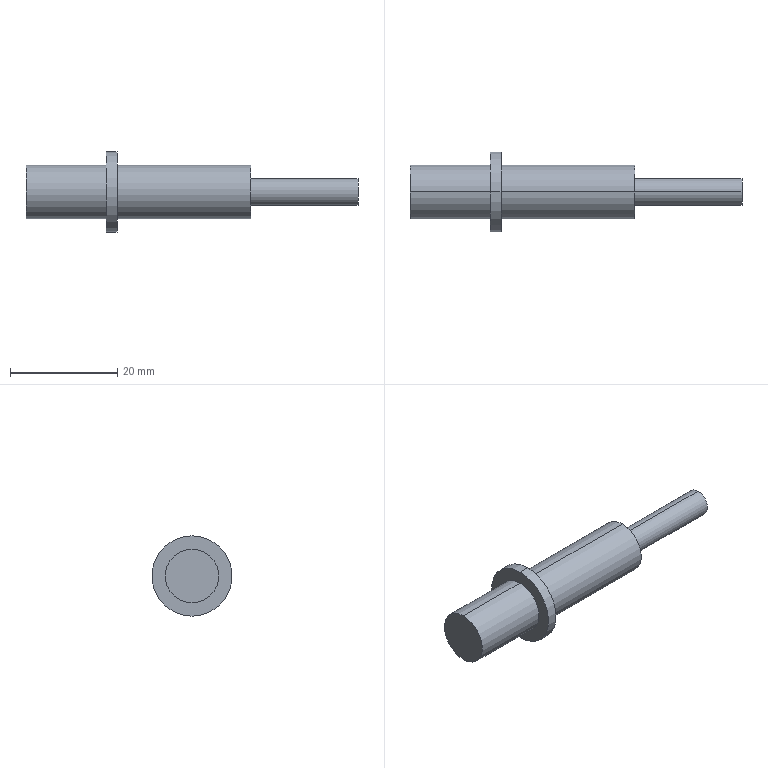Part | SolidWorks | features ICE 3, Extrusion 1 | 1 solid | 13 faces | box 62 x 15 x 15 mm | volume 3888 mm3 | cylinder 8 | plane 5 | commonest cylinder face diameters 10 x4 5 x2 15 x2
STEP:
#1=CARTESIAN_POINT('',(-42.,0.,5.));
#2=VERTEX_POINT('',#1);
#3=CARTESIAN_POINT('',(-42.,0.,-5.));
#4=VERTEX_POINT('',#3);
#5=CARTESIAN_POINT('',(-42.,0.,0.));
#6=DIRECTION('',(-1.,0.,0.));
#7=DIRECTION('',(0.,0.,1.));
#8=AXIS2_PLACEMENT_3D('',#5,#6,#7);
#9=CIRCLE('',#8,5.);
#10=EDGE_CURVE('',#2,#4,#9,.T.);
#11=ORIENTED_EDGE('',*,*,#10,.F.);
#12=CARTESIAN_POINT('',(-27.,0.,5.));
#13=VERTEX_POINT('',#12);
#14=CARTESIAN_POINT('',(-42.,0.,5.));
#15=DIRECTION('',(1.,0.,0.));
#16=VECTOR('',#15,1000.);
#17=LINE('',#14,#16);
#18=EDGE_CURVE('',#2,#13,#17,.T.);
#19=ORIENTED_EDGE('',*,*,#18,.T.);
#20=CARTESIAN_POINT('',(-27.,0.,-5.));
#21=VERTEX_POINT('',#20);
#22=CARTESIAN_POINT('',(-27.,0.,0.));
#23=DIRECTION('',(-1.,0.,0.));
#24=DIRECTION('',(0.,0.,1.));
#25=AXIS2_PLACEMENT_3D('',#22,#23,#24);
#26=CIRCLE('',#25,5.);
#27=EDGE_CURVE('',#13,#21,#26,.T.);
#28=ORIENTED_EDGE('',*,*,#27,.T.);
#29=CARTESIAN_POINT('',(-42.,0.,-5.));
#30=DIRECTION('',(1.,0.,0.));
#31=VECTOR('',#30,1000.);
#32=LINE('',#29,#31);
#33=EDGE_CURVE('',#4,#21,#32,.T.);
#34=ORIENTED_EDGE('',*,*,#33,.F.);
#35=EDGE_LOOP('',(#11,#19,#28,#34));
#36=FACE_OUTER_BOUND('',#35,.T.);
#37=CARTESIAN_POINT('',(-42.,0.,0.));
#38=DIRECTION('',(1.,0.,0.));
#39=DIRECTION('',(0.,0.,-1.));
#40=AXIS2_PLACEMENT_3D('',#37,#38,#39);
#41=CYLINDRICAL_SURFACE('',#40,5.);
#42=ADVANCED_FACE('',(#36),#41,.T.);
#43=CARTESIAN_POINT('',(-27.,0.,7.5));
#44=VERTEX_POINT('',#43);
#45=CARTESIAN_POINT('',(-27.,0.,-7.5));
#46=VERTEX_POINT('',#45);
#47=CARTESIAN_POINT('',(-27.,0.,0.));
#48=DIRECTION('',(-1.,0.,0.));
#49=DIRECTION('',(0.,0.,1.));
#50=AXIS2_PLACEMENT_3D('',#47,#48,#49);
#51=CIRCLE('',#50,7.5);
#52=EDGE_CURVE('',#44,#46,#51,.T.);
#53=ORIENTED_EDGE('',*,*,#52,.F.);
#54=CARTESIAN_POINT('',(-25.,0.,7.5));
#55=VERTEX_POINT('',#54);
#56=CARTESIAN_POINT('',(-27.,0.,7.5));
#57=DIRECTION('',(1.,0.,0.));
#58=VECTOR('',#57,1000.);
#59=LINE('',#56,#58);
#60=EDGE_CURVE('',#44,#55,#59,.T.);
#61=ORIENTED_EDGE('',*,*,#60,.T.);
#62=CARTESIAN_POINT('',(-25.,0.,-7.5));
#63=VERTEX_POINT('',#62);
#64=CARTESIAN_POINT('',(-25.,0.,0.));
#65=DIRECTION('',(-1.,0.,0.));
#66=DIRECTION('',(0.,0.,1.));
#67=AXIS2_PLACEMENT_3D('',#64,#65,#66);
#68=CIRCLE('',#67,7.5);
#69=EDGE_CURVE('',#55,#63,#68,.T.);
#70=ORIENTED_EDGE('',*,*,#69,.T.);
#71=CARTESIAN_POINT('',(-27.,0.,-7.5));
#72=DIRECTION('',(1.,0.,0.));
#73=VECTOR('',#72,1000.);
#74=LINE('',#71,#73);
#75=EDGE_CURVE('',#46,#63,#74,.T.);
#76=ORIENTED_EDGE('',*,*,#75,.F.);
#77=EDGE_LOOP('',(#53,#61,#70,#76));
#78=FACE_OUTER_BOUND('',#77,.T.);
#79=CARTESIAN_POINT('',(-27.,0.,0.));
#80=DIRECTION('',(1.,0.,0.));
#81=DIRECTION('',(0.,0.,-1.));
#82=AXIS2_PLACEMENT_3D('',#79,#80,#81);
#83=CYLINDRICAL_SURFACE('',#82,7.5);
#84=ADVANCED_FACE('',(#78),#83,.T.);
#85=CARTESIAN_POINT('',(-25.,0.,5.));
#86=VERTEX_POINT('',#85);
#87=CARTESIAN_POINT('',(-25.,0.,-5.));
#88=VERTEX_POINT('',#87);
#89=CARTESIAN_POINT('',(-25.,0.,0.));
#90=DIRECTION('',(-1.,0.,0.));
#91=DIRECTION('',(0.,0.,1.));
#92=AXIS2_PLACEMENT_3D('',#89,#90,#91);
#93=CIRCLE('',#92,5.);
#94=EDGE_CURVE('',#86,#88,#93,.T.);
#95=ORIENTED_EDGE('',*,*,#94,.F.);
#96=CARTESIAN_POINT('',(0.,0.,5.));
#97=VERTEX_POINT('',#96);
#98=CARTESIAN_POINT('',(-25.,0.,5.));
#99=DIRECTION('',(1.,0.,0.));
#100=VECTOR('',#99,1000.);
#101=LINE('',#98,#100);
#102=EDGE_CURVE('',#86,#97,#101,.T.);
#103=ORIENTED_EDGE('',*,*,#102,.T.);
#104=CARTESIAN_POINT('',(0.,0.,-5.));
#105=VERTEX_POINT('',#104);
#106=CARTESIAN_POINT('',(0.,0.,0.));
#107=DIRECTION('',(-1.,0.,0.));
#108=DIRECTION('',(0.,0.,1.));
#109=AXIS2_PLACEMENT_3D('',#106,#107,#108);
#110=CIRCLE('',#109,5.);
#111=EDGE_CURVE('',#97,#105,#110,.T.);
#112=ORIENTED_EDGE('',*,*,#111,.T.);
#113=CARTESIAN_POINT('',(-25.,0.,-5.));
#114=DIRECTION('',(1.,0.,0.));
#115=VECTOR('',#114,1000.);
#116=LINE('',#113,#115);
#117=EDGE_CURVE('',#88,#105,#116,.T.);
#118=ORIENTED_EDGE('',*,*,#117,.F.);
#119=EDGE_LOOP('',(#95,#103,#112,#118));
#120=FACE_OUTER_BOUND('',#119,.T.);
#121=CARTESIAN_POINT('',(-25.,0.,0.));
#122=DIRECTION('',(1.,0.,0.));
#123=DIRECTION('',(0.,0.,-1.));
#124=AXIS2_PLACEMENT_3D('',#121,#122,#123);
#125=CYLINDRICAL_SURFACE('',#124,5.);
#126=ADVANCED_FACE('',(#120),#125,.T.);
#127=CARTESIAN_POINT('',(20.,0.,-2.5));
#128=VERTEX_POINT('',#127);
#129=CARTESIAN_POINT('',(20.,0.,2.5));
#130=VERTEX_POINT('',#129);
#131=CARTESIAN_POINT('',(20.,0.,0.));
#132=DIRECTION('',(1.,0.,0.));
#133=DIRECTION('',(0.,0.,-1.));
#134=AXIS2_PLACEMENT_3D('',#131,#132,#133);
#135=CIRCLE('',#134,2.5);
#136=EDGE_CURVE('',#128,#130,#135,.T.);
#137=ORIENTED_EDGE('',*,*,#136,.F.);
#138=CARTESIAN_POINT('',(0.,0.,-2.5));
#139=VERTEX_POINT('',#138);
#140=CARTESIAN_POINT('',(20.,0.,-2.5));
#141=DIRECTION('',(-1.,0.,0.));
#142=VECTOR('',#141,1000.);
#143=LINE('',#140,#142);
#144=EDGE_CURVE('',#128,#139,#143,.T.);
#145=ORIENTED_EDGE('',*,*,#144,.T.);
#146=CARTESIAN_POINT('',(0.,0.,2.5));
#147=VERTEX_POINT('',#146);
#148=CARTESIAN_POINT('',(0.,0.,0.));
#149=DIRECTION('',(1.,0.,0.));
#150=DIRECTION('',(0.,0.,-1.));
#151=AXIS2_PLACEMENT_3D('',#148,#149,#150);
#152=CIRCLE('',#151,2.5);
#153=EDGE_CURVE('',#139,#147,#152,.T.);
#154=ORIENTED_EDGE('',*,*,#153,.T.);
#155=CARTESIAN_POINT('',(20.,0.,2.5));
#156=DIRECTION('',(-1.,0.,0.));
#157=VECTOR('',#156,1000.);
#158=LINE('',#155,#157);
#159=EDGE_CURVE('',#130,#147,#158,.T.);
#160=ORIENTED_EDGE('',*,*,#159,.F.);
#161=EDGE_LOOP('',(#137,#145,#154,#160));
#162=FACE_OUTER_BOUND('',#161,.T.);
#163=CARTESIAN_POINT('',(20.,0.,0.));
#164=DIRECTION('',(-1.,0.,0.));
#165=DIRECTION('',(0.,0.,1.));
#166=AXIS2_PLACEMENT_3D('',#163,#164,#165);
#167=CYLINDRICAL_SURFACE('',#166,2.5);
#168=ADVANCED_FACE('',(#162),#167,.T.);
#169=ORIENTED_EDGE('',*,*,#144,.F.);
#170=CARTESIAN_POINT('',(20.,0.,0.));
#171=DIRECTION('',(1.,0.,0.));
#172=DIRECTION('',(0.,0.,-1.));
#173=AXIS2_PLACEMENT_3D('',#170,#171,#172);
#174=CIRCLE('',#173,2.5);
#175=EDGE_CURVE('',#130,#128,#174,.T.);
#176=ORIENTED_EDGE('',*,*,#175,.F.);
#177=ORIENTED_EDGE('',*,*,#159,.T.);
#178=CARTESIAN_POINT('',(0.,0.,0.));
#179=DIRECTION('',(1.,0.,0.));
#180=DIRECTION('',(0.,0.,-1.));
#181=AXIS2_PLACEMENT_3D('',#178,#179,#180);
#182=CIRCLE('',#181,2.5);
#183=EDGE_CURVE('',#147,#139,#182,.T.);
#184=ORIENTED_EDGE('',*,*,#183,.T.);
#185=EDGE_LOOP('',(#169,#176,#177,#184));
#186=FACE_OUTER_BOUND('',#185,.T.);
#187=CARTESIAN_POINT('',(20.,0.,0.));
#188=DIRECTION('',(-1.,0.,0.));
#189=DIRECTION('',(0.,0.,1.));
#190=AXIS2_PLACEMENT_3D('',#187,#188,#189);
#191=CYLINDRICAL_SURFACE('',#190,2.5);
#192=ADVANCED_FACE('',(#186),#191,.T.);
#193=ORIENTED_EDGE('',*,*,#175,.T.);
#194=ORIENTED_EDGE('',*,*,#136,.T.);
#195=EDGE_LOOP('',(#193,#194));
#196=FACE_OUTER_BOUND('',#195,.T.);
#197=CARTESIAN_POINT('',(20.,0.,0.));
#198=DIRECTION('',(1.,0.,0.));
#199=DIRECTION('',(0.,0.,-1.));
#200=AXIS2_PLACEMENT_3D('',#197,#198,#199);
#201=PLANE('',#200);
#202=ADVANCED_FACE('',(#196),#201,.T.);
#203=ORIENTED_EDGE('',*,*,#102,.F.);
#204=CARTESIAN_POINT('',(-25.,0.,0.));
#205=DIRECTION('',(-1.,0.,0.));
#206=DIRECTION('',(0.,0.,1.));
#207=AXIS2_PLACEMENT_3D('',#204,#205,#206);
#208=CIRCLE('',#207,5.);
#209=EDGE_CURVE('',#88,#86,#208,.T.);
#210=ORIENTED_EDGE('',*,*,#209,.F.);
#211=ORIENTED_EDGE('',*,*,#117,.T.);
#212=CARTESIAN_POINT('',(0.,0.,0.));
#213=DIRECTION('',(-1.,0.,0.));
#214=DIRECTION('',(0.,0.,1.));
#215=AXIS2_PLACEMENT_3D('',#212,#213,#214);
#216=CIRCLE('',#215,5.);
#217=EDGE_CURVE('',#105,#97,#216,.T.);
#218=ORIENTED_EDGE('',*,*,#217,.T.);
#219=EDGE_LOOP('',(#203,#210,#211,#218));
#220=FACE_OUTER_BOUND('',#219,.T.);
#221=CARTESIAN_POINT('',(-25.,0.,0.));
#222=DIRECTION('',(1.,0.,0.));
#223=DIRECTION('',(0.,0.,-1.));
#224=AXIS2_PLACEMENT_3D('',#221,#222,#223);
#225=CYLINDRICAL_SURFACE('',#224,5.);
#226=ADVANCED_FACE('',(#220),#225,.T.);
#227=ORIENTED_EDGE('',*,*,#183,.F.);
#228=ORIENTED_EDGE('',*,*,#153,.F.);
#229=EDGE_LOOP('',(#227,#228));
#230=FACE_BOUND('',#229,.T.);
#231=ORIENTED_EDGE('',*,*,#217,.F.);
#232=ORIENTED_EDGE('',*,*,#111,.F.);
#233=EDGE_LOOP('',(#231,#232));
#234=FACE_OUTER_BOUND('',#233,.T.);
#235=CARTESIAN_POINT('',(0.,0.,0.));
#236=DIRECTION('',(-1.,0.,0.));
#237=DIRECTION('',(0.,0.,1.));
#238=AXIS2_PLACEMENT_3D('',#235,#236,#237);
#239=PLANE('',#238);
#240=ADVANCED_FACE('',(#230,#234),#239,.F.);
#241=ORIENTED_EDGE('',*,*,#60,.F.);
#242=CARTESIAN_POINT('',(-27.,0.,0.));
#243=DIRECTION('',(-1.,0.,0.));
#244=DIRECTION('',(0.,0.,1.));
#245=AXIS2_PLACEMENT_3D('',#242,#243,#244);
#246=CIRCLE('',#245,7.5);
#247=EDGE_CURVE('',#46,#44,#246,.T.);
#248=ORIENTED_EDGE('',*,*,#247,.F.);
#249=ORIENTED_EDGE('',*,*,#75,.T.);
#250=CARTESIAN_POINT('',(-25.,0.,0.));
#251=DIRECTION('',(-1.,0.,0.));
#252=DIRECTION('',(0.,0.,1.));
#253=AXIS2_PLACEMENT_3D('',#250,#251,#252);
#254=CIRCLE('',#253,7.5);
#255=EDGE_CURVE('',#63,#55,#254,.T.);
#256=ORIENTED_EDGE('',*,*,#255,.T.);
#257=EDGE_LOOP('',(#241,#248,#249,#256));
#258=FACE_OUTER_BOUND('',#257,.T.);
#259=CARTESIAN_POINT('',(-27.,0.,0.));
#260=DIRECTION('',(1.,0.,0.));
#261=DIRECTION('',(0.,0.,-1.));
#262=AXIS2_PLACEMENT_3D('',#259,#260,#261);
#263=CYLINDRICAL_SURFACE('',#262,7.5);
#264=ADVANCED_FACE('',(#258),#263,.T.);
#265=CARTESIAN_POINT('',(-27.,0.,0.));
#266=DIRECTION('',(-1.,0.,0.));
#267=DIRECTION('',(0.,0.,1.));
#268=AXIS2_PLACEMENT_3D('',#265,#266,#267);
#269=CIRCLE('',#268,5.);
#270=EDGE_CURVE('',#21,#13,#269,.T.);
#271=ORIENTED_EDGE('',*,*,#270,.F.);
#272=ORIENTED_EDGE('',*,*,#27,.F.);
#273=EDGE_LOOP('',(#271,#272));
#274=FACE_BOUND('',#273,.T.);
#275=ORIENTED_EDGE('',*,*,#247,.T.);
#276=ORIENTED_EDGE('',*,*,#52,.T.);
#277=EDGE_LOOP('',(#275,#276));
#278=FACE_OUTER_BOUND('',#277,.T.);
#279=CARTESIAN_POINT('',(-27.,0.,0.));
#280=DIRECTION('',(-1.,0.,0.));
#281=DIRECTION('',(0.,0.,1.));
#282=AXIS2_PLACEMENT_3D('',#279,#280,#281);
#283=PLANE('',#282);
#284=ADVANCED_FACE('',(#274,#278),#283,.T.);
#285=ORIENTED_EDGE('',*,*,#209,.T.);
#286=ORIENTED_EDGE('',*,*,#94,.T.);
#287=EDGE_LOOP('',(#285,#286));
#288=FACE_BOUND('',#287,.T.);
#289=ORIENTED_EDGE('',*,*,#255,.F.);
#290=ORIENTED_EDGE('',*,*,#69,.F.);
#291=EDGE_LOOP('',(#289,#290));
#292=FACE_OUTER_BOUND('',#291,.T.);
#293=CARTESIAN_POINT('',(-25.,0.,0.));
#294=DIRECTION('',(-1.,0.,0.));
#295=DIRECTION('',(0.,0.,1.));
#296=AXIS2_PLACEMENT_3D('',#293,#294,#295);
#297=PLANE('',#296);
#298=ADVANCED_FACE('',(#288,#292),#297,.F.);
#299=ORIENTED_EDGE('',*,*,#18,.F.);
#300=CARTESIAN_POINT('',(-42.,0.,0.));
#301=DIRECTION('',(-1.,0.,0.));
#302=DIRECTION('',(0.,0.,1.));
#303=AXIS2_PLACEMENT_3D('',#300,#301,#302);
#304=CIRCLE('',#303,5.);
#305=EDGE_CURVE('',#4,#2,#304,.T.);
#306=ORIENTED_EDGE('',*,*,#305,.F.);
#307=ORIENTED_EDGE('',*,*,#33,.T.);
#308=ORIENTED_EDGE('',*,*,#270,.T.);
#309=EDGE_LOOP('',(#299,#306,#307,#308));
#310=FACE_OUTER_BOUND('',#309,.T.);
#311=CARTESIAN_POINT('',(-42.,0.,0.));
#312=DIRECTION('',(1.,0.,0.));
#313=DIRECTION('',(0.,0.,-1.));
#314=AXIS2_PLACEMENT_3D('',#311,#312,#313);
#315=CYLINDRICAL_SURFACE('',#314,5.);
#316=ADVANCED_FACE('',(#310),#315,.T.);
#317=ORIENTED_EDGE('',*,*,#305,.T.);
#318=ORIENTED_EDGE('',*,*,#10,.T.);
#319=EDGE_LOOP('',(#317,#318));
#320=FACE_OUTER_BOUND('',#319,.T.);
#321=CARTESIAN_POINT('',(-42.,0.,0.));
#322=DIRECTION('',(-1.,0.,0.));
#323=DIRECTION('',(0.,0.,1.));
#324=AXIS2_PLACEMENT_3D('',#321,#322,#323);
#325=PLANE('',#324);
#326=ADVANCED_FACE('',(#320),#325,.T.);
#327=CLOSED_SHELL('',(#42,#84,#126,#168,#192,#202,#226,#240,#264,#284,#298,#316,#326));
#328=MANIFOLD_SOLID_BREP('',#327);
#329=CARTESIAN_POINT('',(0.,0.,0.));
#330=DIRECTION('',(0.,0.,1.));
#331=DIRECTION('',(1.,0.,0.));
#332=AXIS2_PLACEMENT_3D('',#329,#330,#331);
#333=(LENGTH_UNIT()NAMED_UNIT(*)SI_UNIT(.MILLI.,.METRE.));
#334=UNCERTAINTY_MEASURE_WITH_UNIT(LENGTH_MEASURE(0.00001),#333,'','');
#335=(NAMED_UNIT(*)PLANE_ANGLE_UNIT()SI_UNIT($,.RADIAN.));
#336=(NAMED_UNIT(*)SI_UNIT($,.STERADIAN.)SOLID_ANGLE_UNIT());
#337=(GEOMETRIC_REPRESENTATION_CONTEXT(3)GLOBAL_UNCERTAINTY_ASSIGNED_CONTEXT((#334))GLOBAL_UNIT_ASSIGNED_CONTEXT((#333,#335,#336))REPRESENTATION_CONTEXT('',''));
#338=ADVANCED_BREP_SHAPE_REPRESENTATION('',(#328,#332),#337);